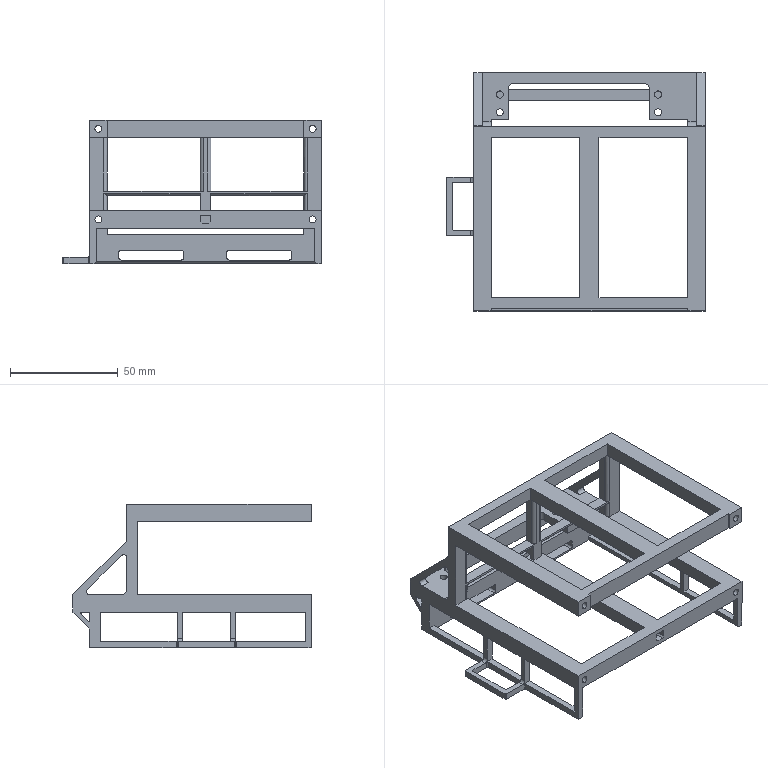Part | SolidWorks | features ICE 28, Chamfer 5, Fillet 5, MirrorPattern 2, Extrusion 1 | 1 solid | 195 faces | box 119.7 x 110.236 x 66.6 mm | volume 59225 mm3 | plane 137 | cylinder 58 | commonest cylinder face diameters 1 x16 3 x14 2 x8 3.2 x8 3.3 x8 4 x2